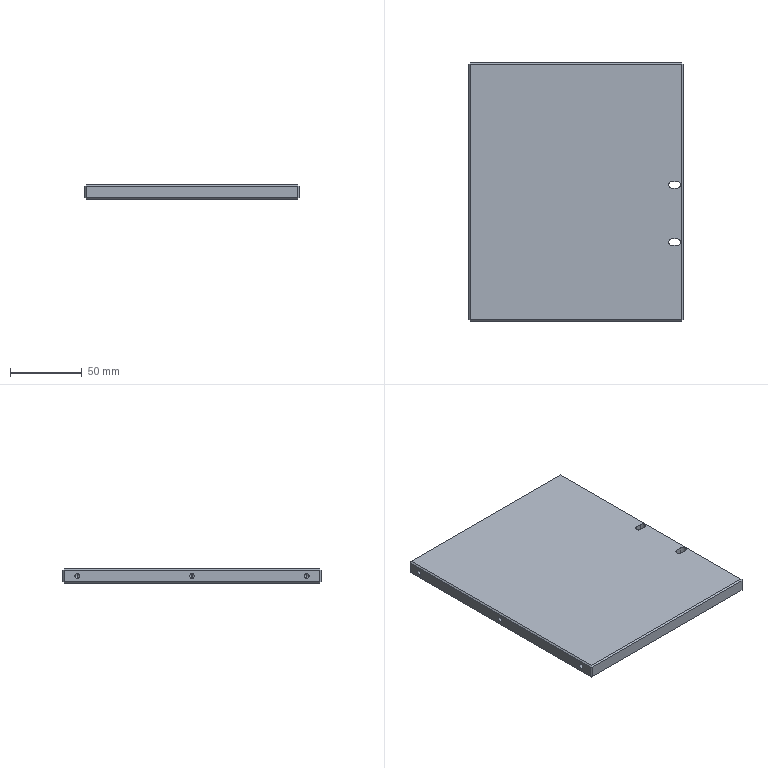Part | STEP file | 01-14 side plate | 1 solid | 48 faces | box 149.5 x 180 x 10 mm | volume 267445 mm3 | plane 30 | cylinder 12 | cone 6 | commonest cylinder face diameters 3.3 x6 4.5 x6
STEP:
#1=CARTESIAN_POINT('',(-62.259,80.,5.));
#2=VERTEX_POINT('',#1);
#3=CARTESIAN_POINT('',(-63.25,80.,6.65));
#4=VERTEX_POINT('',#3);
#5=CARTESIAN_POINT('',(-63.25,80.,6.65));
#6=DIRECTION('',(-0.515,0.,0.8572));
#7=VECTOR('',#6,1000.);
#8=LINE('',#5,#7);
#9=EDGE_CURVE('',#2,#4,#8,.T.);
#10=ORIENTED_EDGE('',*,*,#9,.F.);
#11=CARTESIAN_POINT('',(-63.25,80.,3.35));
#12=VERTEX_POINT('',#11);
#13=CARTESIAN_POINT('',(-63.25,80.,3.35));
#14=DIRECTION('',(-0.515,0.,-0.8572));
#15=VECTOR('',#14,1000.);
#16=LINE('',#13,#15);
#17=EDGE_CURVE('',#2,#12,#16,.T.);
#18=ORIENTED_EDGE('',*,*,#17,.T.);
#19=CARTESIAN_POINT('',(-63.25,80.,5.));
#20=DIRECTION('',(-1.,0.,0.));
#21=DIRECTION('',(0.,0.,1.));
#22=AXIS2_PLACEMENT_3D('',#19,#20,#21);
#23=CIRCLE('',#22,1.65);
#24=EDGE_CURVE('',#12,#4,#23,.T.);
#25=ORIENTED_EDGE('',*,*,#24,.T.);
#26=EDGE_LOOP('',(#10,#18,#25));
#27=FACE_OUTER_BOUND('',#26,.T.);
#28=CARTESIAN_POINT('',(-63.25,80.,5.));
#29=DIRECTION('',(-1.,0.,0.));
#30=DIRECTION('',(0.,0.,1.));
#31=AXIS2_PLACEMENT_3D('',#28,#29,#30);
#32=CONICAL_SURFACE('',#31,1.65,1.03);
#33=ADVANCED_FACE('',(#27),#32,.F.);
#34=ORIENTED_EDGE('',*,*,#24,.F.);
#35=CARTESIAN_POINT('',(-74.75,80.,3.35));
#36=VERTEX_POINT('',#35);
#37=CARTESIAN_POINT('',(-74.75,80.,3.35));
#38=DIRECTION('',(-1.,0.,0.));
#39=VECTOR('',#38,1000.);
#40=LINE('',#37,#39);
#41=EDGE_CURVE('',#12,#36,#40,.T.);
#42=ORIENTED_EDGE('',*,*,#41,.T.);
#43=CARTESIAN_POINT('',(-74.75,80.,6.65));
#44=VERTEX_POINT('',#43);
#45=CARTESIAN_POINT('',(-74.75,80.,5.));
#46=DIRECTION('',(-1.,0.,0.));
#47=DIRECTION('',(0.,0.,1.));
#48=AXIS2_PLACEMENT_3D('',#45,#46,#47);
#49=CIRCLE('',#48,1.65);
#50=EDGE_CURVE('',#36,#44,#49,.T.);
#51=ORIENTED_EDGE('',*,*,#50,.T.);
#52=CARTESIAN_POINT('',(-74.75,80.,6.65));
#53=DIRECTION('',(-1.,0.,0.));
#54=VECTOR('',#53,1000.);
#55=LINE('',#52,#54);
#56=EDGE_CURVE('',#4,#44,#55,.T.);
#57=ORIENTED_EDGE('',*,*,#56,.F.);
#58=EDGE_LOOP('',(#34,#42,#51,#57));
#59=FACE_OUTER_BOUND('',#58,.T.);
#60=CARTESIAN_POINT('',(-74.75,80.,5.));
#61=DIRECTION('',(-1.,0.,0.));
#62=DIRECTION('',(0.,0.,1.));
#63=AXIS2_PLACEMENT_3D('',#60,#61,#62);
#64=CYLINDRICAL_SURFACE('',#63,1.65);
#65=ADVANCED_FACE('',(#59),#64,.F.);
#66=CARTESIAN_POINT('',(-63.25,0.,3.35));
#67=VERTEX_POINT('',#66);
#68=CARTESIAN_POINT('',(-63.25,0.,6.65));
#69=VERTEX_POINT('',#68);
#70=CARTESIAN_POINT('',(-63.25,0.,5.));
#71=DIRECTION('',(-1.,0.,0.));
#72=DIRECTION('',(0.,0.,1.));
#73=AXIS2_PLACEMENT_3D('',#70,#71,#72);
#74=CIRCLE('',#73,1.65);
#75=EDGE_CURVE('',#67,#69,#74,.T.);
#76=ORIENTED_EDGE('',*,*,#75,.F.);
#77=CARTESIAN_POINT('',(-74.75,0.,3.35));
#78=VERTEX_POINT('',#77);
#79=CARTESIAN_POINT('',(-74.75,0.,3.35));
#80=DIRECTION('',(-1.,0.,0.));
#81=VECTOR('',#80,1000.);
#82=LINE('',#79,#81);
#83=EDGE_CURVE('',#67,#78,#82,.T.);
#84=ORIENTED_EDGE('',*,*,#83,.T.);
#85=CARTESIAN_POINT('',(-74.75,0.,6.65));
#86=VERTEX_POINT('',#85);
#87=CARTESIAN_POINT('',(-74.75,0.,5.));
#88=DIRECTION('',(-1.,0.,0.));
#89=DIRECTION('',(0.,0.,1.));
#90=AXIS2_PLACEMENT_3D('',#87,#88,#89);
#91=CIRCLE('',#90,1.65);
#92=EDGE_CURVE('',#78,#86,#91,.T.);
#93=ORIENTED_EDGE('',*,*,#92,.T.);
#94=CARTESIAN_POINT('',(-74.75,0.,6.65));
#95=DIRECTION('',(-1.,0.,0.));
#96=VECTOR('',#95,1000.);
#97=LINE('',#94,#96);
#98=EDGE_CURVE('',#69,#86,#97,.T.);
#99=ORIENTED_EDGE('',*,*,#98,.F.);
#100=EDGE_LOOP('',(#76,#84,#93,#99));
#101=FACE_OUTER_BOUND('',#100,.T.);
#102=CARTESIAN_POINT('',(-74.75,0.,5.));
#103=DIRECTION('',(-1.,0.,0.));
#104=DIRECTION('',(0.,0.,1.));
#105=AXIS2_PLACEMENT_3D('',#102,#103,#104);
#106=CYLINDRICAL_SURFACE('',#105,1.65);
#107=ADVANCED_FACE('',(#101),#106,.F.);
#108=CARTESIAN_POINT('',(-62.259,0.,5.));
#109=VERTEX_POINT('',#108);
#110=CARTESIAN_POINT('',(-63.25,0.,6.65));
#111=DIRECTION('',(-0.515,0.,0.8572));
#112=VECTOR('',#111,1000.);
#113=LINE('',#110,#112);
#114=EDGE_CURVE('',#109,#69,#113,.T.);
#115=ORIENTED_EDGE('',*,*,#114,.F.);
#116=CARTESIAN_POINT('',(-63.25,0.,3.35));
#117=DIRECTION('',(-0.515,0.,-0.8572));
#118=VECTOR('',#117,1000.);
#119=LINE('',#116,#118);
#120=EDGE_CURVE('',#109,#67,#119,.T.);
#121=ORIENTED_EDGE('',*,*,#120,.T.);
#122=ORIENTED_EDGE('',*,*,#75,.T.);
#123=EDGE_LOOP('',(#115,#121,#122));
#124=FACE_OUTER_BOUND('',#123,.T.);
#125=CARTESIAN_POINT('',(-63.25,0.,5.));
#126=DIRECTION('',(-1.,0.,0.));
#127=DIRECTION('',(0.,0.,1.));
#128=AXIS2_PLACEMENT_3D('',#125,#126,#127);
#129=CONICAL_SURFACE('',#128,1.65,1.03);
#130=ADVANCED_FACE('',(#124),#129,.F.);
#131=CARTESIAN_POINT('',(-63.25,-80.,3.35));
#132=VERTEX_POINT('',#131);
#133=CARTESIAN_POINT('',(-63.25,-80.,6.65));
#134=VERTEX_POINT('',#133);
#135=CARTESIAN_POINT('',(-63.25,-80.,5.));
#136=DIRECTION('',(-1.,0.,0.));
#137=DIRECTION('',(0.,0.,1.));
#138=AXIS2_PLACEMENT_3D('',#135,#136,#137);
#139=CIRCLE('',#138,1.65);
#140=EDGE_CURVE('',#132,#134,#139,.T.);
#141=ORIENTED_EDGE('',*,*,#140,.F.);
#142=CARTESIAN_POINT('',(-74.75,-80.,3.35));
#143=VERTEX_POINT('',#142);
#144=CARTESIAN_POINT('',(-74.75,-80.,3.35));
#145=DIRECTION('',(-1.,0.,0.));
#146=VECTOR('',#145,1000.);
#147=LINE('',#144,#146);
#148=EDGE_CURVE('',#132,#143,#147,.T.);
#149=ORIENTED_EDGE('',*,*,#148,.T.);
#150=CARTESIAN_POINT('',(-74.75,-80.,6.65));
#151=VERTEX_POINT('',#150);
#152=CARTESIAN_POINT('',(-74.75,-80.,5.));
#153=DIRECTION('',(-1.,0.,0.));
#154=DIRECTION('',(0.,0.,1.));
#155=AXIS2_PLACEMENT_3D('',#152,#153,#154);
#156=CIRCLE('',#155,1.65);
#157=EDGE_CURVE('',#143,#151,#156,.T.);
#158=ORIENTED_EDGE('',*,*,#157,.T.);
#159=CARTESIAN_POINT('',(-74.75,-80.,6.65));
#160=DIRECTION('',(-1.,0.,0.));
#161=VECTOR('',#160,1000.);
#162=LINE('',#159,#161);
#163=EDGE_CURVE('',#134,#151,#162,.T.);
#164=ORIENTED_EDGE('',*,*,#163,.F.);
#165=EDGE_LOOP('',(#141,#149,#158,#164));
#166=FACE_OUTER_BOUND('',#165,.T.);
#167=CARTESIAN_POINT('',(-74.75,-80.,5.));
#168=DIRECTION('',(-1.,0.,0.));
#169=DIRECTION('',(0.,0.,1.));
#170=AXIS2_PLACEMENT_3D('',#167,#168,#169);
#171=CYLINDRICAL_SURFACE('',#170,1.65);
#172=ADVANCED_FACE('',(#166),#171,.F.);
#173=CARTESIAN_POINT('',(-62.259,-80.,5.));
#174=VERTEX_POINT('',#173);
#175=CARTESIAN_POINT('',(-63.25,-80.,6.65));
#176=DIRECTION('',(-0.515,0.,0.8572));
#177=VECTOR('',#176,1000.);
#178=LINE('',#175,#177);
#179=EDGE_CURVE('',#174,#134,#178,.T.);
#180=ORIENTED_EDGE('',*,*,#179,.F.);
#181=CARTESIAN_POINT('',(-63.25,-80.,3.35));
#182=DIRECTION('',(-0.515,0.,-0.8572));
#183=VECTOR('',#182,1000.);
#184=LINE('',#181,#183);
#185=EDGE_CURVE('',#174,#132,#184,.T.);
#186=ORIENTED_EDGE('',*,*,#185,.T.);
#187=ORIENTED_EDGE('',*,*,#140,.T.);
#188=EDGE_LOOP('',(#180,#186,#187));
#189=FACE_OUTER_BOUND('',#188,.T.);
#190=CARTESIAN_POINT('',(-63.25,-80.,5.));
#191=DIRECTION('',(-1.,0.,0.));
#192=DIRECTION('',(0.,0.,1.));
#193=AXIS2_PLACEMENT_3D('',#190,#191,#192);
#194=CONICAL_SURFACE('',#193,1.65,1.03);
#195=ADVANCED_FACE('',(#189),#194,.F.);
#196=CARTESIAN_POINT('',(73.,-35.,0.));
#197=VERTEX_POINT('',#196);
#198=CARTESIAN_POINT('',(70.75,-32.75,0.));
#199=VERTEX_POINT('',#198);
#200=CARTESIAN_POINT('',(70.75,-35.,0.));
#201=DIRECTION('',(0.,0.,1.));
#202=DIRECTION('',(1.,0.,0.));
#203=AXIS2_PLACEMENT_3D('',#200,#201,#202);
#204=CIRCLE('',#203,2.25);
#205=EDGE_CURVE('',#197,#199,#204,.T.);
#206=ORIENTED_EDGE('',*,*,#205,.F.);
#207=CARTESIAN_POINT('',(73.,-35.,10.));
#208=VERTEX_POINT('',#207);
#209=CARTESIAN_POINT('',(73.,-35.,0.));
#210=DIRECTION('',(0.,0.,1.));
#211=VECTOR('',#210,1000.);
#212=LINE('',#209,#211);
#213=EDGE_CURVE('',#197,#208,#212,.T.);
#214=ORIENTED_EDGE('',*,*,#213,.T.);
#215=CARTESIAN_POINT('',(70.75,-32.75,10.));
#216=VERTEX_POINT('',#215);
#217=CARTESIAN_POINT('',(70.75,-35.,10.));
#218=DIRECTION('',(0.,0.,1.));
#219=DIRECTION('',(1.,0.,0.));
#220=AXIS2_PLACEMENT_3D('',#217,#218,#219);
#221=CIRCLE('',#220,2.25);
#222=EDGE_CURVE('',#208,#216,#221,.T.);
#223=ORIENTED_EDGE('',*,*,#222,.T.);
#224=CARTESIAN_POINT('',(70.75,-32.75,0.));
#225=DIRECTION('',(0.,0.,1.));
#226=VECTOR('',#225,1000.);
#227=LINE('',#224,#226);
#228=EDGE_CURVE('',#199,#216,#227,.T.);
#229=ORIENTED_EDGE('',*,*,#228,.F.);
#230=EDGE_LOOP('',(#206,#214,#223,#229));
#231=FACE_OUTER_BOUND('',#230,.T.);
#232=CARTESIAN_POINT('',(70.75,-35.,0.));
#233=DIRECTION('',(0.,0.,1.));
#234=DIRECTION('',(1.,0.,0.));
#235=AXIS2_PLACEMENT_3D('',#232,#233,#234);
#236=CYLINDRICAL_SURFACE('',#235,2.25);
#237=ADVANCED_FACE('',(#231),#236,.F.);
#238=CARTESIAN_POINT('',(73.,5.,0.));
#239=VERTEX_POINT('',#238);
#240=CARTESIAN_POINT('',(70.75,7.25,0.));
#241=VERTEX_POINT('',#240);
#242=CARTESIAN_POINT('',(70.75,5.,0.));
#243=DIRECTION('',(0.,0.,1.));
#244=DIRECTION('',(1.,0.,0.));
#245=AXIS2_PLACEMENT_3D('',#242,#243,#244);
#246=CIRCLE('',#245,2.25);
#247=EDGE_CURVE('',#239,#241,#246,.T.);
#248=ORIENTED_EDGE('',*,*,#247,.F.);
#249=CARTESIAN_POINT('',(73.,5.,10.));
#250=VERTEX_POINT('',#249);
#251=CARTESIAN_POINT('',(73.,5.,0.));
#252=DIRECTION('',(0.,0.,1.));
#253=VECTOR('',#252,1000.);
#254=LINE('',#251,#253);
#255=EDGE_CURVE('',#239,#250,#254,.T.);
#256=ORIENTED_EDGE('',*,*,#255,.T.);
#257=CARTESIAN_POINT('',(70.75,7.25,10.));
#258=VERTEX_POINT('',#257);
#259=CARTESIAN_POINT('',(70.75,5.,10.));
#260=DIRECTION('',(0.,0.,1.));
#261=DIRECTION('',(1.,0.,0.));
#262=AXIS2_PLACEMENT_3D('',#259,#260,#261);
#263=CIRCLE('',#262,2.25);
#264=EDGE_CURVE('',#250,#258,#263,.T.);
#265=ORIENTED_EDGE('',*,*,#264,.T.);
#266=CARTESIAN_POINT('',(70.75,7.25,0.));
#267=DIRECTION('',(0.,0.,1.));
#268=VECTOR('',#267,1000.);
#269=LINE('',#266,#268);
#270=EDGE_CURVE('',#241,#258,#269,.T.);
#271=ORIENTED_EDGE('',*,*,#270,.F.);
#272=EDGE_LOOP('',(#248,#256,#265,#271));
#273=FACE_OUTER_BOUND('',#272,.T.);
#274=CARTESIAN_POINT('',(70.75,5.,0.));
#275=DIRECTION('',(0.,0.,1.));
#276=DIRECTION('',(1.,0.,0.));
#277=AXIS2_PLACEMENT_3D('',#274,#275,#276);
#278=CYLINDRICAL_SURFACE('',#277,2.25);
#279=ADVANCED_FACE('',(#273),#278,.F.);
#280=CARTESIAN_POINT('',(-74.75,89.,1.));
#281=VERTEX_POINT('',#280);
#282=CARTESIAN_POINT('',(-74.75,-89.,1.));
#283=VERTEX_POINT('',#282);
#284=CARTESIAN_POINT('',(-74.75,90.,1.));
#285=DIRECTION('',(0.,-1.,0.));
#286=VECTOR('',#285,1000.);
#287=LINE('',#284,#286);
#288=EDGE_CURVE('',#281,#283,#287,.T.);
#289=ORIENTED_EDGE('',*,*,#288,.T.);
#290=CARTESIAN_POINT('',(-74.75,-89.,9.));
#291=VERTEX_POINT('',#290);
#292=CARTESIAN_POINT('',(-74.75,-89.,10.));
#293=DIRECTION('',(0.,0.,1.));
#294=VECTOR('',#293,1000.);
#295=LINE('',#292,#294);
#296=EDGE_CURVE('',#283,#291,#295,.T.);
#297=ORIENTED_EDGE('',*,*,#296,.T.);
#298=CARTESIAN_POINT('',(-74.75,89.,9.));
#299=VERTEX_POINT('',#298);
#300=CARTESIAN_POINT('',(-74.75,90.,9.));
#301=DIRECTION('',(0.,1.,0.));
#302=VECTOR('',#301,1000.);
#303=LINE('',#300,#302);
#304=EDGE_CURVE('',#291,#299,#303,.T.);
#305=ORIENTED_EDGE('',*,*,#304,.T.);
#306=CARTESIAN_POINT('',(-74.75,89.,10.));
#307=DIRECTION('',(0.,0.,-1.));
#308=VECTOR('',#307,1000.);
#309=LINE('',#306,#308);
#310=EDGE_CURVE('',#299,#281,#309,.T.);
#311=ORIENTED_EDGE('',*,*,#310,.T.);
#312=EDGE_LOOP('',(#289,#297,#305,#311));
#313=FACE_OUTER_BOUND('',#312,.T.);
#314=CARTESIAN_POINT('',(-74.75,0.,5.));
#315=DIRECTION('',(-1.,0.,0.));
#316=DIRECTION('',(0.,0.,1.));
#317=AXIS2_PLACEMENT_3D('',#314,#315,#316);
#318=CIRCLE('',#317,1.65);
#319=EDGE_CURVE('',#86,#78,#318,.T.);
#320=ORIENTED_EDGE('',*,*,#319,.F.);
#321=ORIENTED_EDGE('',*,*,#92,.F.);
#322=EDGE_LOOP('',(#320,#321));
#323=FACE_BOUND('',#322,.T.);
#324=CARTESIAN_POINT('',(-74.75,-80.,5.));
#325=DIRECTION('',(-1.,0.,0.));
#326=DIRECTION('',(0.,0.,1.));
#327=AXIS2_PLACEMENT_3D('',#324,#325,#326);
#328=CIRCLE('',#327,1.65);
#329=EDGE_CURVE('',#151,#143,#328,.T.);
#330=ORIENTED_EDGE('',*,*,#329,.F.);
#331=ORIENTED_EDGE('',*,*,#157,.F.);
#332=EDGE_LOOP('',(#330,#331));
#333=FACE_BOUND('',#332,.T.);
#334=CARTESIAN_POINT('',(-74.75,80.,5.));
#335=DIRECTION('',(-1.,0.,0.));
#336=DIRECTION('',(0.,0.,1.));
#337=AXIS2_PLACEMENT_3D('',#334,#335,#336);
#338=CIRCLE('',#337,1.65);
#339=EDGE_CURVE('',#44,#36,#338,.T.);
#340=ORIENTED_EDGE('',*,*,#339,.F.);
#341=ORIENTED_EDGE('',*,*,#50,.F.);
#342=EDGE_LOOP('',(#340,#341));
#343=FACE_BOUND('',#342,.T.);
#344=CARTESIAN_POINT('',(-74.75,90.,10.));
#345=DIRECTION('',(1.,0.,0.));
#346=DIRECTION('',(0.,1.,0.));
#347=AXIS2_PLACEMENT_3D('',#344,#345,#346);
#348=PLANE('',#347);
#349=ADVANCED_FACE('',(#313,#323,#333,#343),#348,.F.);
#350=CARTESIAN_POINT('',(74.75,89.,9.));
#351=VERTEX_POINT('',#350);
#352=CARTESIAN_POINT('',(74.75,-89.,9.));
#353=VERTEX_POINT('',#352);
#354=CARTESIAN_POINT('',(74.75,-90.,9.));
#355=DIRECTION('',(0.,-1.,0.));
#356=VECTOR('',#355,1000.);
#357=LINE('',#354,#356);
#358=EDGE_CURVE('',#351,#353,#357,.T.);
#359=ORIENTED_EDGE('',*,*,#358,.T.);
#360=CARTESIAN_POINT('',(74.75,-89.,1.));
#361=VERTEX_POINT('',#360);
#362=CARTESIAN_POINT('',(74.75,-89.,10.));
#363=DIRECTION('',(0.,0.,-1.));
#364=VECTOR('',#363,1000.);
#365=LINE('',#362,#364);
#366=EDGE_CURVE('',#353,#361,#365,.T.);
#367=ORIENTED_EDGE('',*,*,#366,.T.);
#368=CARTESIAN_POINT('',(74.75,89.,1.));
#369=VERTEX_POINT('',#368);
#370=CARTESIAN_POINT('',(74.75,90.,1.));
#371=DIRECTION('',(0.,1.,0.));
#372=VECTOR('',#371,1000.);
#373=LINE('',#370,#372);
#374=EDGE_CURVE('',#361,#369,#373,.T.);
#375=ORIENTED_EDGE('',*,*,#374,.T.);
#376=CARTESIAN_POINT('',(74.75,89.,10.));
#377=DIRECTION('',(0.,0.,1.));
#378=VECTOR('',#377,1000.);
#379=LINE('',#376,#378);
#380=EDGE_CURVE('',#369,#351,#379,.T.);
#381=ORIENTED_EDGE('',*,*,#380,.T.);
#382=EDGE_LOOP('',(#359,#367,#375,#381));
#383=FACE_OUTER_BOUND('',#382,.T.);
#384=CARTESIAN_POINT('',(74.75,90.,10.));
#385=DIRECTION('',(-1.,0.,0.));
#386=DIRECTION('',(0.,-1.,0.));
#387=AXIS2_PLACEMENT_3D('',#384,#385,#386);
#388=PLANE('',#387);
#389=ADVANCED_FACE('',(#383),#388,.F.);
#390=CARTESIAN_POINT('',(-73.75,90.,9.));
#391=VERTEX_POINT('',#390);
#392=CARTESIAN_POINT('',(73.75,90.,9.));
#393=VERTEX_POINT('',#392);
#394=CARTESIAN_POINT('',(74.75,90.,9.));
#395=DIRECTION('',(1.,0.,0.));
#396=VECTOR('',#395,1000.);
#397=LINE('',#394,#396);
#398=EDGE_CURVE('',#391,#393,#397,.T.);
#399=ORIENTED_EDGE('',*,*,#398,.T.);
#400=CARTESIAN_POINT('',(73.75,90.,1.));
#401=VERTEX_POINT('',#400);
#402=CARTESIAN_POINT('',(73.75,90.,10.));
#403=DIRECTION('',(0.,0.,-1.));
#404=VECTOR('',#403,1000.);
#405=LINE('',#402,#404);
#406=EDGE_CURVE('',#393,#401,#405,.T.);
#407=ORIENTED_EDGE('',*,*,#406,.T.);
#408=CARTESIAN_POINT('',(-73.75,90.,1.));
#409=VERTEX_POINT('',#408);
#410=CARTESIAN_POINT('',(-74.75,90.,1.));
#411=DIRECTION('',(-1.,0.,0.));
#412=VECTOR('',#411,1000.);
#413=LINE('',#410,#412);
#414=EDGE_CURVE('',#401,#409,#413,.T.);
#415=ORIENTED_EDGE('',*,*,#414,.T.);
#416=CARTESIAN_POINT('',(-73.75,90.,10.));
#417=DIRECTION('',(0.,0.,1.));
#418=VECTOR('',#417,1000.);
#419=LINE('',#416,#418);
#420=EDGE_CURVE('',#409,#391,#419,.T.);
#421=ORIENTED_EDGE('',*,*,#420,.T.);
#422=EDGE_LOOP('',(#399,#407,#415,#421));
#423=FACE_OUTER_BOUND('',#422,.T.);
#424=CARTESIAN_POINT('',(-74.75,90.,10.));
#425=DIRECTION('',(0.,-1.,0.));
#426=DIRECTION('',(0.,0.,-1.));
#427=AXIS2_PLACEMENT_3D('',#424,#425,#426);
#428=PLANE('',#427);
#429=ADVANCED_FACE('',(#423),#428,.F.);
#430=CARTESIAN_POINT('',(73.75,-90.,9.));
#431=VERTEX_POINT('',#430);
#432=CARTESIAN_POINT('',(-73.75,-90.,9.));
#433=VERTEX_POINT('',#432);
#434=CARTESIAN_POINT('',(-74.75,-90.,9.));
#435=DIRECTION('',(-1.,0.,0.));
#436=VECTOR('',#435,1000.);
#437=LINE('',#434,#436);
#438=EDGE_CURVE('',#431,#433,#437,.T.);
#439=ORIENTED_EDGE('',*,*,#438,.T.);
#440=CARTESIAN_POINT('',(-73.75,-90.,1.));
#441=VERTEX_POINT('',#440);
#442=CARTESIAN_POINT('',(-73.75,-90.,10.));
#443=DIRECTION('',(0.,0.,-1.));
#444=VECTOR('',#443,1000.);
#445=LINE('',#442,#444);
#446=EDGE_CURVE('',#433,#441,#445,.T.);
#447=ORIENTED_EDGE('',*,*,#446,.T.);
#448=CARTESIAN_POINT('',(73.75,-90.,1.));
#449=VERTEX_POINT('',#448);
#450=CARTESIAN_POINT('',(-74.75,-90.,1.));
#451=DIRECTION('',(1.,0.,0.));
#452=VECTOR('',#451,1000.);
#453=LINE('',#450,#452);
#454=EDGE_CURVE('',#441,#449,#453,.T.);
#455=ORIENTED_EDGE('',*,*,#454,.T.);
#456=CARTESIAN_POINT('',(73.75,-90.,10.));
#457=DIRECTION('',(0.,0.,1.));
#458=VECTOR('',#457,1000.);
#459=LINE('',#456,#458);
#460=EDGE_CURVE('',#449,#431,#459,.T.);
#461=ORIENTED_EDGE('',*,*,#460,.T.);
#462=EDGE_LOOP('',(#439,#447,#455,#461));
#463=FACE_OUTER_BOUND('',#462,.T.);
#464=CARTESIAN_POINT('',(-74.75,-90.,10.));
#465=DIRECTION('',(0.,1.,0.));
#466=DIRECTION('',(0.,0.,1.));
#467=AXIS2_PLACEMENT_3D('',#464,#465,#466);
#468=PLANE('',#467);
#469=ADVANCED_FACE('',(#463),#468,.F.);
#470=CARTESIAN_POINT('',(-73.75,-89.,10.));
#471=VERTEX_POINT('',#470);
#472=CARTESIAN_POINT('',(73.75,-89.,10.));
#473=VERTEX_POINT('',#472);
#474=CARTESIAN_POINT('',(74.75,-89.,10.));
#475=DIRECTION('',(1.,0.,0.));
#476=VECTOR('',#475,1000.);
#477=LINE('',#474,#476);
#478=EDGE_CURVE('',#471,#473,#477,.T.);
#479=ORIENTED_EDGE('',*,*,#478,.T.);
#480=CARTESIAN_POINT('',(73.75,89.,10.));
#481=VERTEX_POINT('',#480);
#482=CARTESIAN_POINT('',(73.75,90.,10.));
#483=DIRECTION('',(0.,1.,0.));
#484=VECTOR('',#483,1000.);
#485=LINE('',#482,#484);
#486=EDGE_CURVE('',#473,#481,#485,.T.);
#487=ORIENTED_EDGE('',*,*,#486,.T.);
#488=CARTESIAN_POINT('',(-73.75,89.,10.));
#489=VERTEX_POINT('',#488);
#490=CARTESIAN_POINT('',(-74.75,89.,10.));
#491=DIRECTION('',(-1.,0.,0.));
#492=VECTOR('',#491,1000.);
#493=LINE('',#490,#492);
#494=EDGE_CURVE('',#481,#489,#493,.T.);
#495=ORIENTED_EDGE('',*,*,#494,.T.);
#496=CARTESIAN_POINT('',(-73.75,-90.,10.));
#497=DIRECTION('',(0.,-1.,0.));
#498=VECTOR('',#497,1000.);
#499=LINE('',#496,#498);
#500=EDGE_CURVE('',#489,#471,#499,.T.);
#501=ORIENTED_EDGE('',*,*,#500,.T.);
#502=EDGE_LOOP('',(#479,#487,#495,#501));
#503=FACE_OUTER_BOUND('',#502,.T.);
#504=CARTESIAN_POINT('',(66.75,-32.75,10.));
#505=VERTEX_POINT('',#504);
#506=CARTESIAN_POINT('',(66.75,-37.25,10.));
#507=VERTEX_POINT('',#506);
#508=CARTESIAN_POINT('',(66.75,-35.,10.));
#509=DIRECTION('',(0.,0.,1.));
#510=DIRECTION('',(1.,0.,0.));
#511=AXIS2_PLACEMENT_3D('',#508,#509,#510);
#512=CIRCLE('',#511,2.25);
#513=EDGE_CURVE('',#505,#507,#512,.T.);
#514=ORIENTED_EDGE('',*,*,#513,.F.);
#515=CARTESIAN_POINT('',(66.75,-32.75,10.));
#516=DIRECTION('',(-1.,0.,0.));
#517=VECTOR('',#516,1000.);
#518=LINE('',#515,#517);
#519=EDGE_CURVE('',#216,#505,#518,.T.);
#520=ORIENTED_EDGE('',*,*,#519,.F.);
#521=ORIENTED_EDGE('',*,*,#222,.F.);
#522=CARTESIAN_POINT('',(70.75,-37.25,10.));
#523=VERTEX_POINT('',#522);
#524=CARTESIAN_POINT('',(70.75,-35.,10.));
#525=DIRECTION('',(0.,0.,1.));
#526=DIRECTION('',(1.,0.,0.));
#527=AXIS2_PLACEMENT_3D('',#524,#525,#526);
#528=CIRCLE('',#527,2.25);
#529=EDGE_CURVE('',#523,#208,#528,.T.);
#530=ORIENTED_EDGE('',*,*,#529,.F.);
#531=CARTESIAN_POINT('',(66.75,-37.25,10.));
#532=DIRECTION('',(1.,0.,0.));
#533=VECTOR('',#532,1000.);
#534=LINE('',#531,#533);
#535=EDGE_CURVE('',#507,#523,#534,.T.);
#536=ORIENTED_EDGE('',*,*,#535,.F.);
#537=EDGE_LOOP('',(#514,#520,#521,#530,#536));
#538=FACE_BOUND('',#537,.T.);
#539=CARTESIAN_POINT('',(66.75,7.25,10.));
#540=VERTEX_POINT('',#539);
#541=CARTESIAN_POINT('',(66.75,2.75,10.));
#542=VERTEX_POINT('',#541);
#543=CARTESIAN_POINT('',(66.75,5.,10.));
#544=DIRECTION('',(0.,0.,1.));
#545=DIRECTION('',(1.,0.,0.));
#546=AXIS2_PLACEMENT_3D('',#543,#544,#545);
#547=CIRCLE('',#546,2.25);
#548=EDGE_CURVE('',#540,#542,#547,.T.);
#549=ORIENTED_EDGE('',*,*,#548,.F.);
#550=CARTESIAN_POINT('',(66.75,7.25,10.));
#551=DIRECTION('',(-1.,0.,0.));
#552=VECTOR('',#551,1000.);
#553=LINE('',#550,#552);
#554=EDGE_CURVE('',#258,#540,#553,.T.);
#555=ORIENTED_EDGE('',*,*,#554,.F.);
#556=ORIENTED_EDGE('',*,*,#264,.F.);
#557=CARTESIAN_POINT('',(70.75,2.75,10.));
#558=VERTEX_POINT('',#557);
#559=CARTESIAN_POINT('',(70.75,5.,10.));
#560=DIRECTION('',(0.,0.,1.));
#561=DIRECTION('',(1.,0.,0.));
#562=AXIS2_PLACEMENT_3D('',#559,#560,#561);
#563=CIRCLE('',#562,2.25);
#564=EDGE_CURVE('',#558,#250,#563,.T.);
#565=ORIENTED_EDGE('',*,*,#564,.F.);
#566=CARTESIAN_POINT('',(66.75,2.75,10.));
#567=DIRECTION('',(1.,0.,0.));
#568=VECTOR('',#567,1000.);
#569=LINE('',#566,#568);
#570=EDGE_CURVE('',#542,#558,#569,.T.);
#571=ORIENTED_EDGE('',*,*,#570,.F.);
#572=EDGE_LOOP('',(#549,#555,#556,#565,#571));
#573=FACE_BOUND('',#572,.T.);
#574=CARTESIAN_POINT('',(74.75,-90.,10.));
#575=DIRECTION('',(0.,0.,1.));
#576=DIRECTION('',(1.,0.,0.));
#577=AXIS2_PLACEMENT_3D('',#574,#575,#576);
#578=PLANE('',#577);
#579=ADVANCED_FACE('',(#503,#538,#573),#578,.T.);
#580=CARTESIAN_POINT('',(-73.75,89.,0.));
#581=VERTEX_POINT('',#580);
#582=CARTESIAN_POINT('',(73.75,89.,0.));
#583=VERTEX_POINT('',#582);
#584=CARTESIAN_POINT('',(74.75,89.,0.));
#585=DIRECTION('',(1.,0.,0.));
#586=VECTOR('',#585,1000.);
#587=LINE('',#584,#586);
#588=EDGE_CURVE('',#581,#583,#587,.T.);
#589=ORIENTED_EDGE('',*,*,#588,.T.);
#590=CARTESIAN_POINT('',(73.75,-89.,0.));
#591=VERTEX_POINT('',#590);
#592=CARTESIAN_POINT('',(73.75,-90.,0.));
#593=DIRECTION('',(0.,-1.,0.));
#594=VECTOR('',#593,1000.);
#595=LINE('',#592,#594);
#596=EDGE_CURVE('',#583,#591,#595,.T.);
#597=ORIENTED_EDGE('',*,*,#596,.T.);
#598=CARTESIAN_POINT('',(-73.75,-89.,0.));
#599=VERTEX_POINT('',#598);
#600=CARTESIAN_POINT('',(74.75,-89.,0.));
#601=DIRECTION('',(-1.,0.,0.));
#602=VECTOR('',#601,1000.);
#603=LINE('',#600,#602);
#604=EDGE_CURVE('',#591,#599,#603,.T.);
#605=ORIENTED_EDGE('',*,*,#604,.T.);
#606=CARTESIAN_POINT('',(-73.75,-90.,0.));
#607=DIRECTION('',(0.,1.,0.));
#608=VECTOR('',#607,1000.);
#609=LINE('',#606,#608);
#610=EDGE_CURVE('',#599,#581,#609,.T.);
#611=ORIENTED_EDGE('',*,*,#610,.T.);
#612=EDGE_LOOP('',(#589,#597,#605,#611));
#613=FACE_OUTER_BOUND('',#612,.T.);
#614=CARTESIAN_POINT('',(66.75,-32.75,0.));
#615=VERTEX_POINT('',#614);
#616=CARTESIAN_POINT('',(66.75,-32.75,0.));
#617=DIRECTION('',(-1.,0.,0.));
#618=VECTOR('',#617,1000.);
#619=LINE('',#616,#618);
#620=EDGE_CURVE('',#199,#615,#619,.T.);
#621=ORIENTED_EDGE('',*,*,#620,.T.);
#622=CARTESIAN_POINT('',(66.75,-37.25,0.));
#623=VERTEX_POINT('',#622);
#624=CARTESIAN_POINT('',(66.75,-35.,0.));
#625=DIRECTION('',(0.,0.,1.));
#626=DIRECTION('',(1.,0.,0.));
#627=AXIS2_PLACEMENT_3D('',#624,#625,#626);
#628=CIRCLE('',#627,2.25);
#629=EDGE_CURVE('',#615,#623,#628,.T.);
#630=ORIENTED_EDGE('',*,*,#629,.T.);
#631=CARTESIAN_POINT('',(70.75,-37.25,0.));
#632=VERTEX_POINT('',#631);
#633=CARTESIAN_POINT('',(66.75,-37.25,0.));
#634=DIRECTION('',(1.,0.,0.));
#635=VECTOR('',#634,1000.);
#636=LINE('',#633,#635);
#637=EDGE_CURVE('',#623,#632,#636,.T.);
#638=ORIENTED_EDGE('',*,*,#637,.T.);
#639=CARTESIAN_POINT('',(70.75,-35.,0.));
#640=DIRECTION('',(0.,0.,1.));
#641=DIRECTION('',(1.,0.,0.));
#642=AXIS2_PLACEMENT_3D('',#639,#640,#641);
#643=CIRCLE('',#642,2.25);
#644=EDGE_CURVE('',#632,#197,#643,.T.);
#645=ORIENTED_EDGE('',*,*,#644,.T.);
#646=ORIENTED_EDGE('',*,*,#205,.T.);
#647=EDGE_LOOP('',(#621,#630,#638,#645,#646));
#648=FACE_BOUND('',#647,.T.);
#649=CARTESIAN_POINT('',(66.75,7.25,0.));
#650=VERTEX_POINT('',#649);
#651=CARTESIAN_POINT('',(66.75,7.25,0.));
#652=DIRECTION('',(-1.,0.,0.));
#653=VECTOR('',#652,1000.);
#654=LINE('',#651,#653);
#655=EDGE_CURVE('',#241,#650,#654,.T.);
#656=ORIENTED_EDGE('',*,*,#655,.T.);
#657=CARTESIAN_POINT('',(66.75,2.75,0.));
#658=VERTEX_POINT('',#657);
#659=CARTESIAN_POINT('',(66.75,5.,0.));
#660=DIRECTION('',(0.,0.,1.));
#661=DIRECTION('',(1.,0.,0.));
#662=AXIS2_PLACEMENT_3D('',#659,#660,#661);
#663=CIRCLE('',#662,2.25);
#664=EDGE_CURVE('',#650,#658,#663,.T.);
#665=ORIENTED_EDGE('',*,*,#664,.T.);
#666=CARTESIAN_POINT('',(70.75,2.75,0.));
#667=VERTEX_POINT('',#666);
#668=CARTESIAN_POINT('',(66.75,2.75,0.));
#669=DIRECTION('',(1.,0.,0.));
#670=VECTOR('',#669,1000.);
#671=LINE('',#668,#670);
#672=EDGE_CURVE('',#658,#667,#671,.T.);
#673=ORIENTED_EDGE('',*,*,#672,.T.);
#674=CARTESIAN_POINT('',(70.75,5.,0.));
#675=DIRECTION('',(0.,0.,1.));
#676=DIRECTION('',(1.,0.,0.));
#677=AXIS2_PLACEMENT_3D('',#674,#675,#676);
#678=CIRCLE('',#677,2.25);
#679=EDGE_CURVE('',#667,#239,#678,.T.);
#680=ORIENTED_EDGE('',*,*,#679,.T.);
#681=ORIENTED_EDGE('',*,*,#247,.T.);
#682=EDGE_LOOP('',(#656,#665,#673,#680,#681));
#683=FACE_BOUND('',#682,.T.);
#684=CARTESIAN_POINT('',(74.75,-90.,0.));
#685=DIRECTION('',(0.,0.,1.));
#686=DIRECTION('',(1.,0.,0.));
#687=AXIS2_PLACEMENT_3D('',#684,#685,#686);
#688=PLANE('',#687);
#689=ADVANCED_FACE('',(#613,#648,#683),#688,.F.);
#690=ORIENTED_EDGE('',*,*,#548,.T.);
#691=CARTESIAN_POINT('',(66.75,2.75,0.));
#692=DIRECTION('',(0.,0.,1.));
#693=VECTOR('',#692,1000.);
#694=LINE('',#691,#693);
#695=EDGE_CURVE('',#658,#542,#694,.T.);
#696=ORIENTED_EDGE('',*,*,#695,.F.);
#697=ORIENTED_EDGE('',*,*,#664,.F.);
#698=CARTESIAN_POINT('',(66.75,7.25,0.));
#699=DIRECTION('',(0.,0.,1.));
#700=VECTOR('',#699,1000.);
#701=LINE('',#698,#700);
#702=EDGE_CURVE('',#650,#540,#701,.T.);
#703=ORIENTED_EDGE('',*,*,#702,.T.);
#704=EDGE_LOOP('',(#690,#696,#697,#703));
#705=FACE_OUTER_BOUND('',#704,.T.);
#706=CARTESIAN_POINT('',(66.75,5.,0.));
#707=DIRECTION('',(0.,0.,1.));
#708=DIRECTION('',(1.,0.,0.));
#709=AXIS2_PLACEMENT_3D('',#706,#707,#708);
#710=CYLINDRICAL_SURFACE('',#709,2.25);
#711=ADVANCED_FACE('',(#705),#710,.F.);
#712=ORIENTED_EDGE('',*,*,#554,.T.);
#713=ORIENTED_EDGE('',*,*,#702,.F.);
#714=ORIENTED_EDGE('',*,*,#655,.F.);
#715=ORIENTED_EDGE('',*,*,#270,.T.);
#716=EDGE_LOOP('',(#712,#713,#714,#715));
#717=FACE_OUTER_BOUND('',#716,.T.);
#718=CARTESIAN_POINT('',(66.75,7.25,0.));
#719=DIRECTION('',(0.,1.,0.));
#720=DIRECTION('',(-1.,0.,0.));
#721=AXIS2_PLACEMENT_3D('',#718,#719,#720);
#722=PLANE('',#721);
#723=ADVANCED_FACE('',(#717),#722,.F.);
#724=ORIENTED_EDGE('',*,*,#255,.F.);
#725=ORIENTED_EDGE('',*,*,#679,.F.);
#726=CARTESIAN_POINT('',(70.75,2.75,0.));
#727=DIRECTION('',(0.,0.,1.));
#728=VECTOR('',#727,1000.);
#729=LINE('',#726,#728);
#730=EDGE_CURVE('',#667,#558,#729,.T.);
#731=ORIENTED_EDGE('',*,*,#730,.T.);
#732=ORIENTED_EDGE('',*,*,#564,.T.);
#733=EDGE_LOOP('',(#724,#725,#731,#732));
#734=FACE_OUTER_BOUND('',#733,.T.);
#735=CARTESIAN_POINT('',(70.75,5.,0.));
#736=DIRECTION('',(0.,0.,1.));
#737=DIRECTION('',(1.,0.,0.));
#738=AXIS2_PLACEMENT_3D('',#735,#736,#737);
#739=CYLINDRICAL_SURFACE('',#738,2.25);
#740=ADVANCED_FACE('',(#734),#739,.F.);
#741=ORIENTED_EDGE('',*,*,#570,.T.);
#742=ORIENTED_EDGE('',*,*,#730,.F.);
#743=ORIENTED_EDGE('',*,*,#672,.F.);
#744=ORIENTED_EDGE('',*,*,#695,.T.);
#745=EDGE_LOOP('',(#741,#742,#743,#744));
#746=FACE_OUTER_BOUND('',#745,.T.);
#747=CARTESIAN_POINT('',(66.75,2.75,0.));
#748=DIRECTION('',(0.,-1.,0.));
#749=DIRECTION('',(1.,0.,0.));
#750=AXIS2_PLACEMENT_3D('',#747,#748,#749);
#751=PLANE('',#750);
#752=ADVANCED_FACE('',(#746),#751,.F.);
#753=ORIENTED_EDGE('',*,*,#513,.T.);
#754=CARTESIAN_POINT('',(66.75,-37.25,0.));
#755=DIRECTION('',(0.,0.,1.));
#756=VECTOR('',#755,1000.);
#757=LINE('',#754,#756);
#758=EDGE_CURVE('',#623,#507,#757,.T.);
#759=ORIENTED_EDGE('',*,*,#758,.F.);
#760=ORIENTED_EDGE('',*,*,#629,.F.);
#761=CARTESIAN_POINT('',(66.75,-32.75,0.));
#762=DIRECTION('',(0.,0.,1.));
#763=VECTOR('',#762,1000.);
#764=LINE('',#761,#763);
#765=EDGE_CURVE('',#615,#505,#764,.T.);
#766=ORIENTED_EDGE('',*,*,#765,.T.);
#767=EDGE_LOOP('',(#753,#759,#760,#766));
#768=FACE_OUTER_BOUND('',#767,.T.);
#769=CARTESIAN_POINT('',(66.75,-35.,0.));
#770=DIRECTION('',(0.,0.,1.));
#771=DIRECTION('',(1.,0.,0.));
#772=AXIS2_PLACEMENT_3D('',#769,#770,#771);
#773=CYLINDRICAL_SURFACE('',#772,2.25);
#774=ADVANCED_FACE('',(#768),#773,.F.);
#775=ORIENTED_EDGE('',*,*,#519,.T.);
#776=ORIENTED_EDGE('',*,*,#765,.F.);
#777=ORIENTED_EDGE('',*,*,#620,.F.);
#778=ORIENTED_EDGE('',*,*,#228,.T.);
#779=EDGE_LOOP('',(#775,#776,#777,#778));
#780=FACE_OUTER_BOUND('',#779,.T.);
#781=CARTESIAN_POINT('',(66.75,-32.75,0.));
#782=DIRECTION('',(0.,1.,0.));
#783=DIRECTION('',(-1.,0.,0.));
#784=AXIS2_PLACEMENT_3D('',#781,#782,#783);
#785=PLANE('',#784);
#786=ADVANCED_FACE('',(#780),#785,.F.);
#787=ORIENTED_EDGE('',*,*,#213,.F.);
#788=ORIENTED_EDGE('',*,*,#644,.F.);
#789=CARTESIAN_POINT('',(70.75,-37.25,0.));
#790=DIRECTION('',(0.,0.,1.));
#791=VECTOR('',#790,1000.);
#792=LINE('',#789,#791);
#793=EDGE_CURVE('',#632,#523,#792,.T.);
#794=ORIENTED_EDGE('',*,*,#793,.T.);
#795=ORIENTED_EDGE('',*,*,#529,.T.);
#796=EDGE_LOOP('',(#787,#788,#794,#795));
#797=FACE_OUTER_BOUND('',#796,.T.);
#798=CARTESIAN_POINT('',(70.75,-35.,0.));
#799=DIRECTION('',(0.,0.,1.));
#800=DIRECTION('',(1.,0.,0.));
#801=AXIS2_PLACEMENT_3D('',#798,#799,#800);
#802=CYLINDRICAL_SURFACE('',#801,2.25);
#803=ADVANCED_FACE('',(#797),#802,.F.);
#804=ORIENTED_EDGE('',*,*,#535,.T.);
#805=ORIENTED_EDGE('',*,*,#793,.F.);
#806=ORIENTED_EDGE('',*,*,#637,.F.);
#807=ORIENTED_EDGE('',*,*,#758,.T.);
#808=EDGE_LOOP('',(#804,#805,#806,#807));
#809=FACE_OUTER_BOUND('',#808,.T.);
#810=CARTESIAN_POINT('',(66.75,-37.25,0.));
#811=DIRECTION('',(0.,-1.,0.));
#812=DIRECTION('',(1.,0.,0.));
#813=AXIS2_PLACEMENT_3D('',#810,#811,#812);
#814=PLANE('',#813);
#815=ADVANCED_FACE('',(#809),#814,.F.);
#816=ORIENTED_EDGE('',*,*,#185,.F.);
#817=ORIENTED_EDGE('',*,*,#179,.T.);
#818=CARTESIAN_POINT('',(-63.25,-80.,5.));
#819=DIRECTION('',(-1.,0.,0.));
#820=DIRECTION('',(0.,0.,1.));
#821=AXIS2_PLACEMENT_3D('',#818,#819,#820);
#822=CIRCLE('',#821,1.65);
#823=EDGE_CURVE('',#134,#132,#822,.T.);
#824=ORIENTED_EDGE('',*,*,#823,.T.);
#825=EDGE_LOOP('',(#816,#817,#824));
#826=FACE_OUTER_BOUND('',#825,.T.);
#827=CARTESIAN_POINT('',(-63.25,-80.,5.));
#828=DIRECTION('',(-1.,0.,0.));
#829=DIRECTION('',(0.,0.,1.));
#830=AXIS2_PLACEMENT_3D('',#827,#828,#829);
#831=CONICAL_SURFACE('',#830,1.65,1.03);
#832=ADVANCED_FACE('',(#826),#831,.F.);
#833=ORIENTED_EDGE('',*,*,#148,.F.);
#834=ORIENTED_EDGE('',*,*,#823,.F.);
#835=ORIENTED_EDGE('',*,*,#163,.T.);
#836=ORIENTED_EDGE('',*,*,#329,.T.);
#837=EDGE_LOOP('',(#833,#834,#835,#836));
#838=FACE_OUTER_BOUND('',#837,.T.);
#839=CARTESIAN_POINT('',(-74.75,-80.,5.));
#840=DIRECTION('',(-1.,0.,0.));
#841=DIRECTION('',(0.,0.,1.));
#842=AXIS2_PLACEMENT_3D('',#839,#840,#841);
#843=CYLINDRICAL_SURFACE('',#842,1.65);
#844=ADVANCED_FACE('',(#838),#843,.F.);
#845=ORIENTED_EDGE('',*,*,#120,.F.);
#846=ORIENTED_EDGE('',*,*,#114,.T.);
#847=CARTESIAN_POINT('',(-63.25,0.,5.));
#848=DIRECTION('',(-1.,0.,0.));
#849=DIRECTION('',(0.,0.,1.));
#850=AXIS2_PLACEMENT_3D('',#847,#848,#849);
#851=CIRCLE('',#850,1.65);
#852=EDGE_CURVE('',#69,#67,#851,.T.);
#853=ORIENTED_EDGE('',*,*,#852,.T.);
#854=EDGE_LOOP('',(#845,#846,#853));
#855=FACE_OUTER_BOUND('',#854,.T.);
#856=CARTESIAN_POINT('',(-63.25,0.,5.));
#857=DIRECTION('',(-1.,0.,0.));
#858=DIRECTION('',(0.,0.,1.));
#859=AXIS2_PLACEMENT_3D('',#856,#857,#858);
#860=CONICAL_SURFACE('',#859,1.65,1.03);
#861=ADVANCED_FACE('',(#855),#860,.F.);
#862=ORIENTED_EDGE('',*,*,#83,.F.);
#863=ORIENTED_EDGE('',*,*,#852,.F.);
#864=ORIENTED_EDGE('',*,*,#98,.T.);
#865=ORIENTED_EDGE('',*,*,#319,.T.);
#866=EDGE_LOOP('',(#862,#863,#864,#865));
#867=FACE_OUTER_BOUND('',#866,.T.);
#868=CARTESIAN_POINT('',(-74.75,0.,5.));
#869=DIRECTION('',(-1.,0.,0.));
#870=DIRECTION('',(0.,0.,1.));
#871=AXIS2_PLACEMENT_3D('',#868,#869,#870);
#872=CYLINDRICAL_SURFACE('',#871,1.65);
#873=ADVANCED_FACE('',(#867),#872,.F.);
#874=ORIENTED_EDGE('',*,*,#41,.F.);
#875=CARTESIAN_POINT('',(-63.25,80.,5.));
#876=DIRECTION('',(-1.,0.,0.));
#877=DIRECTION('',(0.,0.,1.));
#878=AXIS2_PLACEMENT_3D('',#875,#876,#877);
#879=CIRCLE('',#878,1.65);
#880=EDGE_CURVE('',#4,#12,#879,.T.);
#881=ORIENTED_EDGE('',*,*,#880,.F.);
#882=ORIENTED_EDGE('',*,*,#56,.T.);
#883=ORIENTED_EDGE('',*,*,#339,.T.);
#884=EDGE_LOOP('',(#874,#881,#882,#883));
#885=FACE_OUTER_BOUND('',#884,.T.);
#886=CARTESIAN_POINT('',(-74.75,80.,5.));
#887=DIRECTION('',(-1.,0.,0.));
#888=DIRECTION('',(0.,0.,1.));
#889=AXIS2_PLACEMENT_3D('',#886,#887,#888);
#890=CYLINDRICAL_SURFACE('',#889,1.65);
#891=ADVANCED_FACE('',(#885),#890,.F.);
#892=ORIENTED_EDGE('',*,*,#17,.F.);
#893=ORIENTED_EDGE('',*,*,#9,.T.);
#894=ORIENTED_EDGE('',*,*,#880,.T.);
#895=EDGE_LOOP('',(#892,#893,#894));
#896=FACE_OUTER_BOUND('',#895,.T.);
#897=CARTESIAN_POINT('',(-63.25,80.,5.));
#898=DIRECTION('',(-1.,0.,0.));
#899=DIRECTION('',(0.,0.,1.));
#900=AXIS2_PLACEMENT_3D('',#897,#898,#899);
#901=CONICAL_SURFACE('',#900,1.65,1.03);
#902=ADVANCED_FACE('',(#896),#901,.F.);
#903=CARTESIAN_POINT('',(-74.25,-89.,0.5));
#904=DIRECTION('',(0.7071,0.,-0.7071));
#905=VECTOR('',#904,1000.);
#906=LINE('',#903,#905);
#907=EDGE_CURVE('',#283,#599,#906,.T.);
#908=ORIENTED_EDGE('',*,*,#907,.F.);
#909=ORIENTED_EDGE('',*,*,#288,.F.);
#910=CARTESIAN_POINT('',(-74.75,89.,1.));
#911=DIRECTION('',(-0.7071,0.,0.7071));
#912=VECTOR('',#911,1000.);
#913=LINE('',#910,#912);
#914=EDGE_CURVE('',#581,#281,#913,.T.);
#915=ORIENTED_EDGE('',*,*,#914,.F.);
#916=ORIENTED_EDGE('',*,*,#610,.F.);
#917=EDGE_LOOP('',(#908,#909,#915,#916));
#918=FACE_OUTER_BOUND('',#917,.T.);
#919=CARTESIAN_POINT('',(-74.75,90.,1.));
#920=DIRECTION('',(0.7071,0.,0.7071));
#921=DIRECTION('',(0.7071,0.,-0.7071));
#922=AXIS2_PLACEMENT_3D('',#919,#920,#921);
#923=PLANE('',#922);
#924=ADVANCED_FACE('',(#918),#923,.F.);
#925=CARTESIAN_POINT('',(-73.75,-90.,1.));
#926=DIRECTION('',(0.7071,-0.7071,0.));
#927=VECTOR('',#926,1000.);
#928=LINE('',#925,#927);
#929=EDGE_CURVE('',#283,#441,#928,.T.);
#930=ORIENTED_EDGE('',*,*,#929,.F.);
#931=ORIENTED_EDGE('',*,*,#907,.T.);
#932=CARTESIAN_POINT('',(-73.75,-90.,1.));
#933=DIRECTION('',(0.,0.7071,-0.7071));
#934=VECTOR('',#933,1000.);
#935=LINE('',#932,#934);
#936=EDGE_CURVE('',#441,#599,#935,.T.);
#937=ORIENTED_EDGE('',*,*,#936,.F.);
#938=EDGE_LOOP('',(#930,#931,#937));
#939=FACE_OUTER_BOUND('',#938,.T.);
#940=CARTESIAN_POINT('',(-73.75,-90.,1.));
#941=DIRECTION('',(-0.5774,-0.5774,-0.5774));
#942=DIRECTION('',(0.,0.7071,-0.7071));
#943=AXIS2_PLACEMENT_3D('',#940,#941,#942);
#944=PLANE('',#943);
#945=ADVANCED_FACE('',(#939),#944,.T.);
#946=CARTESIAN_POINT('',(-73.75,89.5,0.5));
#947=DIRECTION('',(0.,0.7071,0.7071));
#948=VECTOR('',#947,1000.);
#949=LINE('',#946,#948);
#950=EDGE_CURVE('',#581,#409,#949,.T.);
#951=ORIENTED_EDGE('',*,*,#950,.F.);
#952=ORIENTED_EDGE('',*,*,#914,.T.);
#953=CARTESIAN_POINT('',(-74.75,89.,1.));
#954=DIRECTION('',(-0.7071,-0.7071,0.));
#955=VECTOR('',#954,1000.);
#956=LINE('',#953,#955);
#957=EDGE_CURVE('',#409,#281,#956,.T.);
#958=ORIENTED_EDGE('',*,*,#957,.F.);
#959=EDGE_LOOP('',(#951,#952,#958));
#960=FACE_OUTER_BOUND('',#959,.T.);
#961=CARTESIAN_POINT('',(-74.75,89.,1.));
#962=DIRECTION('',(-0.5774,0.5774,-0.5774));
#963=DIRECTION('',(0.,0.7071,0.7071));
#964=AXIS2_PLACEMENT_3D('',#961,#962,#963);
#965=PLANE('',#964);
#966=ADVANCED_FACE('',(#960),#965,.T.);
#967=ORIENTED_EDGE('',*,*,#936,.T.);
#968=ORIENTED_EDGE('',*,*,#604,.F.);
#969=CARTESIAN_POINT('',(73.75,-89.,0.));
#970=DIRECTION('',(0.,0.7071,-0.7071));
#971=VECTOR('',#970,1000.);
#972=LINE('',#969,#971);
#973=EDGE_CURVE('',#449,#591,#972,.T.);
#974=ORIENTED_EDGE('',*,*,#973,.F.);
#975=ORIENTED_EDGE('',*,*,#454,.F.);
#976=EDGE_LOOP('',(#967,#968,#974,#975));
#977=FACE_OUTER_BOUND('',#976,.T.);
#978=CARTESIAN_POINT('',(-74.75,-90.,1.));
#979=DIRECTION('',(0.,0.7071,0.7071));
#980=DIRECTION('',(0.,-0.7071,0.7071));
#981=AXIS2_PLACEMENT_3D('',#978,#979,#980);
#982=PLANE('',#981);
#983=ADVANCED_FACE('',(#977),#982,.F.);
#984=ORIENTED_EDGE('',*,*,#929,.T.);
#985=ORIENTED_EDGE('',*,*,#446,.F.);
#986=CARTESIAN_POINT('',(-74.75,-89.,9.));
#987=DIRECTION('',(0.7071,-0.7071,0.));
#988=VECTOR('',#987,1000.);
#989=LINE('',#986,#988);
#990=EDGE_CURVE('',#291,#433,#989,.T.);
#991=ORIENTED_EDGE('',*,*,#990,.F.);
#992=ORIENTED_EDGE('',*,*,#296,.F.);
#993=EDGE_LOOP('',(#984,#985,#991,#992));
#994=FACE_OUTER_BOUND('',#993,.T.);
#995=CARTESIAN_POINT('',(-73.75,-90.,10.));
#996=DIRECTION('',(0.7071,0.7071,0.));
#997=DIRECTION('',(-0.7071,0.7071,0.));
#998=AXIS2_PLACEMENT_3D('',#995,#996,#997);
#999=PLANE('',#998);
#1000=ADVANCED_FACE('',(#994),#999,.F.);
#1001=CARTESIAN_POINT('',(-73.75,89.,10.));
#1002=DIRECTION('',(0.7071,0.,0.7071));
#1003=VECTOR('',#1002,1000.);
#1004=LINE('',#1001,#1003);
#1005=EDGE_CURVE('',#299,#489,#1004,.T.);
#1006=ORIENTED_EDGE('',*,*,#1005,.F.);
#1007=ORIENTED_EDGE('',*,*,#304,.F.);
#1008=CARTESIAN_POINT('',(-74.75,-89.,9.));
#1009=DIRECTION('',(-0.7071,0.,-0.7071));
#1010=VECTOR('',#1009,1000.);
#1011=LINE('',#1008,#1010);
#1012=EDGE_CURVE('',#471,#291,#1011,.T.);
#1013=ORIENTED_EDGE('',*,*,#1012,.F.);
#1014=ORIENTED_EDGE('',*,*,#500,.F.);
#1015=EDGE_LOOP('',(#1006,#1007,#1013,#1014));
#1016=FACE_OUTER_BOUND('',#1015,.T.);
#1017=CARTESIAN_POINT('',(-73.75,-90.,10.));
#1018=DIRECTION('',(-0.7071,0.,0.7071));
#1019=DIRECTION('',(0.7071,0.,0.7071));
#1020=AXIS2_PLACEMENT_3D('',#1017,#1018,#1019);
#1021=PLANE('',#1020);
#1022=ADVANCED_FACE('',(#1016),#1021,.T.);
#1023=ORIENTED_EDGE('',*,*,#957,.T.);
#1024=ORIENTED_EDGE('',*,*,#310,.F.);
#1025=CARTESIAN_POINT('',(-74.25,89.5,9.));
#1026=DIRECTION('',(-0.7071,-0.7071,0.));
#1027=VECTOR('',#1026,1000.);
#1028=LINE('',#1025,#1027);
#1029=EDGE_CURVE('',#391,#299,#1028,.T.);
#1030=ORIENTED_EDGE('',*,*,#1029,.F.);
#1031=ORIENTED_EDGE('',*,*,#420,.F.);
#1032=EDGE_LOOP('',(#1023,#1024,#1030,#1031));
#1033=FACE_OUTER_BOUND('',#1032,.T.);
#1034=CARTESIAN_POINT('',(-74.75,89.,10.));
#1035=DIRECTION('',(0.7071,-0.7071,0.));
#1036=DIRECTION('',(0.7071,0.7071,0.));
#1037=AXIS2_PLACEMENT_3D('',#1034,#1035,#1036);
#1038=PLANE('',#1037);
#1039=ADVANCED_FACE('',(#1033),#1038,.F.);
#1040=ORIENTED_EDGE('',*,*,#950,.T.);
#1041=ORIENTED_EDGE('',*,*,#414,.F.);
#1042=CARTESIAN_POINT('',(73.75,89.5,0.5));
#1043=DIRECTION('',(0.,0.7071,0.7071));
#1044=VECTOR('',#1043,1000.);
#1045=LINE('',#1042,#1044);
#1046=EDGE_CURVE('',#583,#401,#1045,.T.);
#1047=ORIENTED_EDGE('',*,*,#1046,.F.);
#1048=ORIENTED_EDGE('',*,*,#588,.F.);
#1049=EDGE_LOOP('',(#1040,#1041,#1047,#1048));
#1050=FACE_OUTER_BOUND('',#1049,.T.);
#1051=CARTESIAN_POINT('',(-74.75,90.,1.));
#1052=DIRECTION('',(0.,-0.7071,0.7071));
#1053=DIRECTION('',(0.,-0.7071,-0.7071));
#1054=AXIS2_PLACEMENT_3D('',#1051,#1052,#1053);
#1055=PLANE('',#1054);
#1056=ADVANCED_FACE('',(#1050),#1055,.F.);
#1057=CARTESIAN_POINT('',(73.75,-89.,0.));
#1058=DIRECTION('',(0.7071,0.,0.7071));
#1059=VECTOR('',#1058,1000.);
#1060=LINE('',#1057,#1059);
#1061=EDGE_CURVE('',#591,#361,#1060,.T.);
#1062=ORIENTED_EDGE('',*,*,#1061,.F.);
#1063=ORIENTED_EDGE('',*,*,#596,.F.);
#1064=CARTESIAN_POINT('',(74.75,89.,1.));
#1065=DIRECTION('',(-0.7071,0.,-0.7071));
#1066=VECTOR('',#1065,1000.);
#1067=LINE('',#1064,#1066);
#1068=EDGE_CURVE('',#369,#583,#1067,.T.);
#1069=ORIENTED_EDGE('',*,*,#1068,.F.);
#1070=ORIENTED_EDGE('',*,*,#374,.F.);
#1071=EDGE_LOOP('',(#1062,#1063,#1069,#1070));
#1072=FACE_OUTER_BOUND('',#1071,.T.);
#1073=CARTESIAN_POINT('',(74.75,90.,1.));
#1074=DIRECTION('',(-0.7071,0.,0.7071));
#1075=DIRECTION('',(0.7071,0.,0.7071));
#1076=AXIS2_PLACEMENT_3D('',#1073,#1074,#1075);
#1077=PLANE('',#1076);
#1078=ADVANCED_FACE('',(#1072),#1077,.F.);
#1079=ORIENTED_EDGE('',*,*,#973,.T.);
#1080=ORIENTED_EDGE('',*,*,#1061,.T.);
#1081=CARTESIAN_POINT('',(74.25,-89.5,1.));
#1082=DIRECTION('',(0.7071,0.7071,0.));
#1083=VECTOR('',#1082,1000.);
#1084=LINE('',#1081,#1083);
#1085=EDGE_CURVE('',#449,#361,#1084,.T.);
#1086=ORIENTED_EDGE('',*,*,#1085,.F.);
#1087=EDGE_LOOP('',(#1079,#1080,#1086));
#1088=FACE_OUTER_BOUND('',#1087,.T.);
#1089=CARTESIAN_POINT('',(73.75,-89.,0.));
#1090=DIRECTION('',(0.5774,-0.5774,-0.5774));
#1091=DIRECTION('',(0.,0.7071,-0.7071));
#1092=AXIS2_PLACEMENT_3D('',#1089,#1090,#1091);
#1093=PLANE('',#1092);
#1094=ADVANCED_FACE('',(#1088),#1093,.T.);
#1095=ORIENTED_EDGE('',*,*,#1012,.T.);
#1096=ORIENTED_EDGE('',*,*,#990,.T.);
#1097=CARTESIAN_POINT('',(-73.75,-89.5,9.5));
#1098=DIRECTION('',(0.,-0.7071,-0.7071));
#1099=VECTOR('',#1098,1000.);
#1100=LINE('',#1097,#1099);
#1101=EDGE_CURVE('',#471,#433,#1100,.T.);
#1102=ORIENTED_EDGE('',*,*,#1101,.F.);
#1103=EDGE_LOOP('',(#1095,#1096,#1102));
#1104=FACE_OUTER_BOUND('',#1103,.T.);
#1105=CARTESIAN_POINT('',(-74.75,-89.,9.));
#1106=DIRECTION('',(-0.5774,-0.5774,0.5774));
#1107=DIRECTION('',(0.,-0.7071,-0.7071));
#1108=AXIS2_PLACEMENT_3D('',#1105,#1106,#1107);
#1109=PLANE('',#1108);
#1110=ADVANCED_FACE('',(#1104),#1109,.T.);
#1111=ORIENTED_EDGE('',*,*,#1029,.T.);
#1112=ORIENTED_EDGE('',*,*,#1005,.T.);
#1113=CARTESIAN_POINT('',(-73.75,89.,10.));
#1114=DIRECTION('',(0.,-0.7071,0.7071));
#1115=VECTOR('',#1114,1000.);
#1116=LINE('',#1113,#1115);
#1117=EDGE_CURVE('',#391,#489,#1116,.T.);
#1118=ORIENTED_EDGE('',*,*,#1117,.F.);
#1119=EDGE_LOOP('',(#1111,#1112,#1118));
#1120=FACE_OUTER_BOUND('',#1119,.T.);
#1121=CARTESIAN_POINT('',(-73.75,89.,10.));
#1122=DIRECTION('',(-0.5774,0.5774,0.5774));
#1123=DIRECTION('',(0.,-0.7071,0.7071));
#1124=AXIS2_PLACEMENT_3D('',#1121,#1122,#1123);
#1125=PLANE('',#1124);
#1126=ADVANCED_FACE('',(#1120),#1125,.T.);
#1127=ORIENTED_EDGE('',*,*,#1068,.T.);
#1128=ORIENTED_EDGE('',*,*,#1046,.T.);
#1129=CARTESIAN_POINT('',(74.75,89.,1.));
#1130=DIRECTION('',(-0.7071,0.7071,0.));
#1131=VECTOR('',#1130,1000.);
#1132=LINE('',#1129,#1131);
#1133=EDGE_CURVE('',#369,#401,#1132,.T.);
#1134=ORIENTED_EDGE('',*,*,#1133,.F.);
#1135=EDGE_LOOP('',(#1127,#1128,#1134));
#1136=FACE_OUTER_BOUND('',#1135,.T.);
#1137=CARTESIAN_POINT('',(74.75,89.,1.));
#1138=DIRECTION('',(0.5774,0.5774,-0.5774));
#1139=DIRECTION('',(-0.7071,0.,-0.7071));
#1140=AXIS2_PLACEMENT_3D('',#1137,#1138,#1139);
#1141=PLANE('',#1140);
#1142=ADVANCED_FACE('',(#1136),#1141,.T.);
#1143=ORIENTED_EDGE('',*,*,#1085,.T.);
#1144=ORIENTED_EDGE('',*,*,#366,.F.);
#1145=CARTESIAN_POINT('',(74.75,-89.,9.));
#1146=DIRECTION('',(0.7071,0.7071,0.));
#1147=VECTOR('',#1146,1000.);
#1148=LINE('',#1145,#1147);
#1149=EDGE_CURVE('',#431,#353,#1148,.T.);
#1150=ORIENTED_EDGE('',*,*,#1149,.F.);
#1151=ORIENTED_EDGE('',*,*,#460,.F.);
#1152=EDGE_LOOP('',(#1143,#1144,#1150,#1151));
#1153=FACE_OUTER_BOUND('',#1152,.T.);
#1154=CARTESIAN_POINT('',(74.75,-89.,10.));
#1155=DIRECTION('',(-0.7071,0.7071,0.));
#1156=DIRECTION('',(-0.7071,-0.7071,0.));
#1157=AXIS2_PLACEMENT_3D('',#1154,#1155,#1156);
#1158=PLANE('',#1157);
#1159=ADVANCED_FACE('',(#1153),#1158,.F.);
#1160=ORIENTED_EDGE('',*,*,#1101,.T.);
#1161=ORIENTED_EDGE('',*,*,#438,.F.);
#1162=CARTESIAN_POINT('',(73.75,-89.5,9.5));
#1163=DIRECTION('',(0.,-0.7071,-0.7071));
#1164=VECTOR('',#1163,1000.);
#1165=LINE('',#1162,#1164);
#1166=EDGE_CURVE('',#473,#431,#1165,.T.);
#1167=ORIENTED_EDGE('',*,*,#1166,.F.);
#1168=ORIENTED_EDGE('',*,*,#478,.F.);
#1169=EDGE_LOOP('',(#1160,#1161,#1167,#1168));
#1170=FACE_OUTER_BOUND('',#1169,.T.);
#1171=CARTESIAN_POINT('',(74.75,-89.,10.));
#1172=DIRECTION('',(0.,-0.7071,0.7071));
#1173=DIRECTION('',(0.,-0.7071,-0.7071));
#1174=AXIS2_PLACEMENT_3D('',#1171,#1172,#1173);
#1175=PLANE('',#1174);
#1176=ADVANCED_FACE('',(#1170),#1175,.T.);
#1177=ORIENTED_EDGE('',*,*,#1117,.T.);
#1178=ORIENTED_EDGE('',*,*,#494,.F.);
#1179=CARTESIAN_POINT('',(73.75,89.,10.));
#1180=DIRECTION('',(0.,-0.7071,0.7071));
#1181=VECTOR('',#1180,1000.);
#1182=LINE('',#1179,#1181);
#1183=EDGE_CURVE('',#393,#481,#1182,.T.);
#1184=ORIENTED_EDGE('',*,*,#1183,.F.);
#1185=ORIENTED_EDGE('',*,*,#398,.F.);
#1186=EDGE_LOOP('',(#1177,#1178,#1184,#1185));
#1187=FACE_OUTER_BOUND('',#1186,.T.);
#1188=CARTESIAN_POINT('',(74.75,89.,10.));
#1189=DIRECTION('',(0.,0.7071,0.7071));
#1190=DIRECTION('',(0.,-0.7071,0.7071));
#1191=AXIS2_PLACEMENT_3D('',#1188,#1189,#1190);
#1192=PLANE('',#1191);
#1193=ADVANCED_FACE('',(#1187),#1192,.T.);
#1194=ORIENTED_EDGE('',*,*,#1133,.T.);
#1195=ORIENTED_EDGE('',*,*,#406,.F.);
#1196=CARTESIAN_POINT('',(74.25,89.5,9.));
#1197=DIRECTION('',(-0.7071,0.7071,0.));
#1198=VECTOR('',#1197,1000.);
#1199=LINE('',#1196,#1198);
#1200=EDGE_CURVE('',#351,#393,#1199,.T.);
#1201=ORIENTED_EDGE('',*,*,#1200,.F.);
#1202=ORIENTED_EDGE('',*,*,#380,.F.);
#1203=EDGE_LOOP('',(#1194,#1195,#1201,#1202));
#1204=FACE_OUTER_BOUND('',#1203,.T.);
#1205=CARTESIAN_POINT('',(73.75,90.,10.));
#1206=DIRECTION('',(-0.7071,-0.7071,0.));
#1207=DIRECTION('',(0.7071,-0.7071,0.));
#1208=AXIS2_PLACEMENT_3D('',#1205,#1206,#1207);
#1209=PLANE('',#1208);
#1210=ADVANCED_FACE('',(#1204),#1209,.F.);
#1211=ORIENTED_EDGE('',*,*,#1166,.T.);
#1212=ORIENTED_EDGE('',*,*,#1149,.T.);
#1213=CARTESIAN_POINT('',(74.75,-89.,9.));
#1214=DIRECTION('',(0.7071,0.,-0.7071));
#1215=VECTOR('',#1214,1000.);
#1216=LINE('',#1213,#1215);
#1217=EDGE_CURVE('',#473,#353,#1216,.T.);
#1218=ORIENTED_EDGE('',*,*,#1217,.F.);
#1219=EDGE_LOOP('',(#1211,#1212,#1218));
#1220=FACE_OUTER_BOUND('',#1219,.T.);
#1221=CARTESIAN_POINT('',(74.75,-89.,9.));
#1222=DIRECTION('',(0.5774,-0.5774,0.5774));
#1223=DIRECTION('',(0.7071,0.7071,0.));
#1224=AXIS2_PLACEMENT_3D('',#1221,#1222,#1223);
#1225=PLANE('',#1224);
#1226=ADVANCED_FACE('',(#1220),#1225,.T.);
#1227=ORIENTED_EDGE('',*,*,#1200,.T.);
#1228=ORIENTED_EDGE('',*,*,#1183,.T.);
#1229=CARTESIAN_POINT('',(73.75,89.,10.));
#1230=DIRECTION('',(-0.7071,0.,0.7071));
#1231=VECTOR('',#1230,1000.);
#1232=LINE('',#1229,#1231);
#1233=EDGE_CURVE('',#351,#481,#1232,.T.);
#1234=ORIENTED_EDGE('',*,*,#1233,.F.);
#1235=EDGE_LOOP('',(#1227,#1228,#1234));
#1236=FACE_OUTER_BOUND('',#1235,.T.);
#1237=CARTESIAN_POINT('',(73.75,89.,10.));
#1238=DIRECTION('',(0.5774,0.5774,0.5774));
#1239=DIRECTION('',(-0.7071,0.7071,0.));
#1240=AXIS2_PLACEMENT_3D('',#1237,#1238,#1239);
#1241=PLANE('',#1240);
#1242=ADVANCED_FACE('',(#1236),#1241,.T.);
#1243=ORIENTED_EDGE('',*,*,#1217,.T.);
#1244=ORIENTED_EDGE('',*,*,#358,.F.);
#1245=ORIENTED_EDGE('',*,*,#1233,.T.);
#1246=ORIENTED_EDGE('',*,*,#486,.F.);
#1247=EDGE_LOOP('',(#1243,#1244,#1245,#1246));
#1248=FACE_OUTER_BOUND('',#1247,.T.);
#1249=CARTESIAN_POINT('',(73.75,-90.,10.));
#1250=DIRECTION('',(0.7071,0.,0.7071));
#1251=DIRECTION('',(0.7071,0.,-0.7071));
#1252=AXIS2_PLACEMENT_3D('',#1249,#1250,#1251);
#1253=PLANE('',#1252);
#1254=ADVANCED_FACE('',(#1248),#1253,.T.);
#1255=CLOSED_SHELL('',(#33,#65,#107,#130,#172,#195,#237,#279,#349,#389,#429,#469,#579,#689,#711,#723,#740,#752,#774,#786,#803,#815,#832,#844,#861,#873,#891,#902,#924,#945,#966,#983,#1000,#1022,#1039,#1056,#1078,#1094,#1110,#1126,#1142,#1159,#1176,#1193,#1210,#1226,#1242,#1254));
#1256=MANIFOLD_SOLID_BREP('',#1255);
#1257=CARTESIAN_POINT('',(0.,0.,0.));
#1258=DIRECTION('',(0.,0.,1.));
#1259=DIRECTION('',(1.,0.,0.));
#1260=AXIS2_PLACEMENT_3D('',#1257,#1258,#1259);
#1261=(LENGTH_UNIT()NAMED_UNIT(*)SI_UNIT(.MILLI.,.METRE.));
#1262=UNCERTAINTY_MEASURE_WITH_UNIT(LENGTH_MEASURE(0.00001),#1261,'','');
#1263=(NAMED_UNIT(*)PLANE_ANGLE_UNIT()SI_UNIT($,.RADIAN.));
#1264=(NAMED_UNIT(*)SI_UNIT($,.STERADIAN.)SOLID_ANGLE_UNIT());
#1265=(GEOMETRIC_REPRESENTATION_CONTEXT(3)GLOBAL_UNCERTAINTY_ASSIGNED_CONTEXT((#1262))GLOBAL_UNIT_ASSIGNED_CONTEXT((#1261,#1263,#1264))REPRESENTATION_CONTEXT('',''));
#1266=ADVANCED_BREP_SHAPE_REPRESENTATION('',(#1256,#1260),#1265);